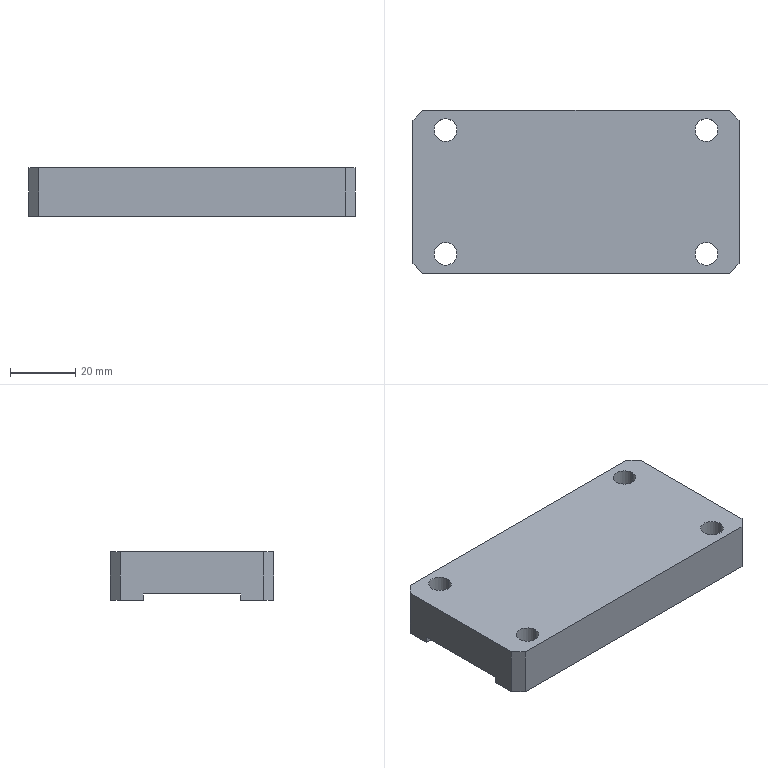Part | SolidWorks | features Chamfer 1, Extrusion 1, HoleWzd 1, ICE 1 | 1 solid | 22 faces | box 100 x 50 x 15 mm | volume 66421 mm3 | plane 14 | cylinder 8 | commonest cylinder face diameters 7 x8
STEP:
#1=CARTESIAN_POINT('',(13.5,44.,15.));
#2=VERTEX_POINT('',#1);
#3=CARTESIAN_POINT('',(6.5,44.,15.));
#4=VERTEX_POINT('',#3);
#5=CARTESIAN_POINT('',(10.,44.,15.));
#6=DIRECTION('',(0.,0.,-1.));
#7=DIRECTION('',(-1.,0.,0.));
#8=AXIS2_PLACEMENT_3D('',#5,#6,#7);
#9=CIRCLE('',#8,3.5);
#10=EDGE_CURVE('',#2,#4,#9,.T.);
#11=ORIENTED_EDGE('',*,*,#10,.F.);
#12=CARTESIAN_POINT('',(13.5,44.,0.));
#13=VERTEX_POINT('',#12);
#14=CARTESIAN_POINT('',(13.5,44.,0.));
#15=DIRECTION('',(0.,0.,-1.));
#16=VECTOR('',#15,1000.);
#17=LINE('',#14,#16);
#18=EDGE_CURVE('',#2,#13,#17,.T.);
#19=ORIENTED_EDGE('',*,*,#18,.T.);
#20=CARTESIAN_POINT('',(6.5,44.,0.));
#21=VERTEX_POINT('',#20);
#22=CARTESIAN_POINT('',(10.,44.,0.));
#23=DIRECTION('',(0.,0.,-1.));
#24=DIRECTION('',(-1.,0.,0.));
#25=AXIS2_PLACEMENT_3D('',#22,#23,#24);
#26=CIRCLE('',#25,3.5);
#27=EDGE_CURVE('',#13,#21,#26,.T.);
#28=ORIENTED_EDGE('',*,*,#27,.T.);
#29=CARTESIAN_POINT('',(6.5,44.,0.));
#30=DIRECTION('',(0.,0.,-1.));
#31=VECTOR('',#30,1000.);
#32=LINE('',#29,#31);
#33=EDGE_CURVE('',#4,#21,#32,.T.);
#34=ORIENTED_EDGE('',*,*,#33,.F.);
#35=EDGE_LOOP('',(#11,#19,#28,#34));
#36=FACE_OUTER_BOUND('',#35,.T.);
#37=CARTESIAN_POINT('',(10.,44.,0.));
#38=DIRECTION('',(0.,0.,-1.));
#39=DIRECTION('',(-1.,0.,0.));
#40=AXIS2_PLACEMENT_3D('',#37,#38,#39);
#41=CYLINDRICAL_SURFACE('',#40,3.5);
#42=ADVANCED_FACE('',(#36),#41,.F.);
#43=CARTESIAN_POINT('',(13.5,6.,15.));
#44=VERTEX_POINT('',#43);
#45=CARTESIAN_POINT('',(6.5,6.,15.));
#46=VERTEX_POINT('',#45);
#47=CARTESIAN_POINT('',(10.,6.,15.));
#48=DIRECTION('',(0.,0.,-1.));
#49=DIRECTION('',(-1.,0.,0.));
#50=AXIS2_PLACEMENT_3D('',#47,#48,#49);
#51=CIRCLE('',#50,3.5);
#52=EDGE_CURVE('',#44,#46,#51,.T.);
#53=ORIENTED_EDGE('',*,*,#52,.F.);
#54=CARTESIAN_POINT('',(13.5,6.,0.));
#55=VERTEX_POINT('',#54);
#56=CARTESIAN_POINT('',(13.5,6.,0.));
#57=DIRECTION('',(0.,0.,-1.));
#58=VECTOR('',#57,1000.);
#59=LINE('',#56,#58);
#60=EDGE_CURVE('',#44,#55,#59,.T.);
#61=ORIENTED_EDGE('',*,*,#60,.T.);
#62=CARTESIAN_POINT('',(6.5,6.,0.));
#63=VERTEX_POINT('',#62);
#64=CARTESIAN_POINT('',(10.,6.,0.));
#65=DIRECTION('',(0.,0.,-1.));
#66=DIRECTION('',(-1.,0.,0.));
#67=AXIS2_PLACEMENT_3D('',#64,#65,#66);
#68=CIRCLE('',#67,3.5);
#69=EDGE_CURVE('',#55,#63,#68,.T.);
#70=ORIENTED_EDGE('',*,*,#69,.T.);
#71=CARTESIAN_POINT('',(6.5,6.,0.));
#72=DIRECTION('',(0.,0.,-1.));
#73=VECTOR('',#72,1000.);
#74=LINE('',#71,#73);
#75=EDGE_CURVE('',#46,#63,#74,.T.);
#76=ORIENTED_EDGE('',*,*,#75,.F.);
#77=EDGE_LOOP('',(#53,#61,#70,#76));
#78=FACE_OUTER_BOUND('',#77,.T.);
#79=CARTESIAN_POINT('',(10.,6.,0.));
#80=DIRECTION('',(0.,0.,-1.));
#81=DIRECTION('',(-1.,0.,0.));
#82=AXIS2_PLACEMENT_3D('',#79,#80,#81);
#83=CYLINDRICAL_SURFACE('',#82,3.5);
#84=ADVANCED_FACE('',(#78),#83,.F.);
#85=CARTESIAN_POINT('',(93.5,44.,15.));
#86=VERTEX_POINT('',#85);
#87=CARTESIAN_POINT('',(86.5,44.,15.));
#88=VERTEX_POINT('',#87);
#89=CARTESIAN_POINT('',(90.,44.,15.));
#90=DIRECTION('',(0.,0.,-1.));
#91=DIRECTION('',(-1.,0.,0.));
#92=AXIS2_PLACEMENT_3D('',#89,#90,#91);
#93=CIRCLE('',#92,3.5);
#94=EDGE_CURVE('',#86,#88,#93,.T.);
#95=ORIENTED_EDGE('',*,*,#94,.F.);
#96=CARTESIAN_POINT('',(93.5,44.,0.));
#97=VERTEX_POINT('',#96);
#98=CARTESIAN_POINT('',(93.5,44.,0.));
#99=DIRECTION('',(0.,0.,-1.));
#100=VECTOR('',#99,1000.);
#101=LINE('',#98,#100);
#102=EDGE_CURVE('',#86,#97,#101,.T.);
#103=ORIENTED_EDGE('',*,*,#102,.T.);
#104=CARTESIAN_POINT('',(86.5,44.,0.));
#105=VERTEX_POINT('',#104);
#106=CARTESIAN_POINT('',(90.,44.,0.));
#107=DIRECTION('',(0.,0.,-1.));
#108=DIRECTION('',(-1.,0.,0.));
#109=AXIS2_PLACEMENT_3D('',#106,#107,#108);
#110=CIRCLE('',#109,3.5);
#111=EDGE_CURVE('',#97,#105,#110,.T.);
#112=ORIENTED_EDGE('',*,*,#111,.T.);
#113=CARTESIAN_POINT('',(86.5,44.,0.));
#114=DIRECTION('',(0.,0.,-1.));
#115=VECTOR('',#114,1000.);
#116=LINE('',#113,#115);
#117=EDGE_CURVE('',#88,#105,#116,.T.);
#118=ORIENTED_EDGE('',*,*,#117,.F.);
#119=EDGE_LOOP('',(#95,#103,#112,#118));
#120=FACE_OUTER_BOUND('',#119,.T.);
#121=CARTESIAN_POINT('',(90.,44.,0.));
#122=DIRECTION('',(0.,0.,-1.));
#123=DIRECTION('',(-1.,0.,0.));
#124=AXIS2_PLACEMENT_3D('',#121,#122,#123);
#125=CYLINDRICAL_SURFACE('',#124,3.5);
#126=ADVANCED_FACE('',(#120),#125,.F.);
#127=CARTESIAN_POINT('',(93.5,6.,15.));
#128=VERTEX_POINT('',#127);
#129=CARTESIAN_POINT('',(86.5,6.,15.));
#130=VERTEX_POINT('',#129);
#131=CARTESIAN_POINT('',(90.,6.,15.));
#132=DIRECTION('',(0.,0.,-1.));
#133=DIRECTION('',(-1.,0.,0.));
#134=AXIS2_PLACEMENT_3D('',#131,#132,#133);
#135=CIRCLE('',#134,3.5);
#136=EDGE_CURVE('',#128,#130,#135,.T.);
#137=ORIENTED_EDGE('',*,*,#136,.F.);
#138=CARTESIAN_POINT('',(93.5,6.,0.));
#139=VERTEX_POINT('',#138);
#140=CARTESIAN_POINT('',(93.5,6.,0.));
#141=DIRECTION('',(0.,0.,-1.));
#142=VECTOR('',#141,1000.);
#143=LINE('',#140,#142);
#144=EDGE_CURVE('',#128,#139,#143,.T.);
#145=ORIENTED_EDGE('',*,*,#144,.T.);
#146=CARTESIAN_POINT('',(86.5,6.,0.));
#147=VERTEX_POINT('',#146);
#148=CARTESIAN_POINT('',(90.,6.,0.));
#149=DIRECTION('',(0.,0.,-1.));
#150=DIRECTION('',(-1.,0.,0.));
#151=AXIS2_PLACEMENT_3D('',#148,#149,#150);
#152=CIRCLE('',#151,3.5);
#153=EDGE_CURVE('',#139,#147,#152,.T.);
#154=ORIENTED_EDGE('',*,*,#153,.T.);
#155=CARTESIAN_POINT('',(86.5,6.,0.));
#156=DIRECTION('',(0.,0.,-1.));
#157=VECTOR('',#156,1000.);
#158=LINE('',#155,#157);
#159=EDGE_CURVE('',#130,#147,#158,.T.);
#160=ORIENTED_EDGE('',*,*,#159,.F.);
#161=EDGE_LOOP('',(#137,#145,#154,#160));
#162=FACE_OUTER_BOUND('',#161,.T.);
#163=CARTESIAN_POINT('',(90.,6.,0.));
#164=DIRECTION('',(0.,0.,-1.));
#165=DIRECTION('',(-1.,0.,0.));
#166=AXIS2_PLACEMENT_3D('',#163,#164,#165);
#167=CYLINDRICAL_SURFACE('',#166,3.5);
#168=ADVANCED_FACE('',(#162),#167,.F.);
#169=CARTESIAN_POINT('',(0.,40.,0.));
#170=VERTEX_POINT('',#169);
#171=CARTESIAN_POINT('',(100.,40.,0.));
#172=VERTEX_POINT('',#171);
#173=CARTESIAN_POINT('',(0.,40.,0.));
#174=DIRECTION('',(1.,0.,0.));
#175=VECTOR('',#174,1000.);
#176=LINE('',#173,#175);
#177=EDGE_CURVE('',#170,#172,#176,.T.);
#178=ORIENTED_EDGE('',*,*,#177,.F.);
#179=CARTESIAN_POINT('',(0.,47.,0.));
#180=VERTEX_POINT('',#179);
#181=CARTESIAN_POINT('',(0.,0.,0.));
#182=DIRECTION('',(0.,-1.,0.));
#183=VECTOR('',#182,1000.);
#184=LINE('',#181,#183);
#185=EDGE_CURVE('',#180,#170,#184,.T.);
#186=ORIENTED_EDGE('',*,*,#185,.F.);
#187=CARTESIAN_POINT('',(3.,50.,0.));
#188=VERTEX_POINT('',#187);
#189=CARTESIAN_POINT('',(-23.5,23.5,0.));
#190=DIRECTION('',(0.7071,0.7071,0.));
#191=VECTOR('',#190,1000.);
#192=LINE('',#189,#191);
#193=EDGE_CURVE('',#180,#188,#192,.T.);
#194=ORIENTED_EDGE('',*,*,#193,.T.);
#195=CARTESIAN_POINT('',(97.,50.,0.));
#196=VERTEX_POINT('',#195);
#197=CARTESIAN_POINT('',(0.,50.,0.));
#198=DIRECTION('',(-1.,0.,0.));
#199=VECTOR('',#198,1000.);
#200=LINE('',#197,#199);
#201=EDGE_CURVE('',#196,#188,#200,.T.);
#202=ORIENTED_EDGE('',*,*,#201,.F.);
#203=CARTESIAN_POINT('',(100.,47.,0.));
#204=VERTEX_POINT('',#203);
#205=CARTESIAN_POINT('',(73.5,73.5,0.));
#206=DIRECTION('',(0.7071,-0.7071,0.));
#207=VECTOR('',#206,1000.);
#208=LINE('',#205,#207);
#209=EDGE_CURVE('',#196,#204,#208,.T.);
#210=ORIENTED_EDGE('',*,*,#209,.T.);
#211=CARTESIAN_POINT('',(100.,0.,0.));
#212=DIRECTION('',(0.,1.,0.));
#213=VECTOR('',#212,1000.);
#214=LINE('',#211,#213);
#215=EDGE_CURVE('',#172,#204,#214,.T.);
#216=ORIENTED_EDGE('',*,*,#215,.F.);
#217=EDGE_LOOP('',(#178,#186,#194,#202,#210,#216));
#218=FACE_OUTER_BOUND('',#217,.T.);
#219=CARTESIAN_POINT('',(90.,44.,0.));
#220=DIRECTION('',(0.,0.,-1.));
#221=DIRECTION('',(-1.,0.,0.));
#222=AXIS2_PLACEMENT_3D('',#219,#220,#221);
#223=CIRCLE('',#222,3.5);
#224=EDGE_CURVE('',#105,#97,#223,.T.);
#225=ORIENTED_EDGE('',*,*,#224,.F.);
#226=ORIENTED_EDGE('',*,*,#111,.F.);
#227=EDGE_LOOP('',(#225,#226));
#228=FACE_BOUND('',#227,.T.);
#229=CARTESIAN_POINT('',(10.,44.,0.));
#230=DIRECTION('',(0.,0.,-1.));
#231=DIRECTION('',(-1.,0.,0.));
#232=AXIS2_PLACEMENT_3D('',#229,#230,#231);
#233=CIRCLE('',#232,3.5);
#234=EDGE_CURVE('',#21,#13,#233,.T.);
#235=ORIENTED_EDGE('',*,*,#234,.F.);
#236=ORIENTED_EDGE('',*,*,#27,.F.);
#237=EDGE_LOOP('',(#235,#236));
#238=FACE_BOUND('',#237,.T.);
#239=CARTESIAN_POINT('',(0.,0.,0.));
#240=DIRECTION('',(0.,0.,-1.));
#241=DIRECTION('',(-1.,0.,0.));
#242=AXIS2_PLACEMENT_3D('',#239,#240,#241);
#243=PLANE('',#242);
#244=ADVANCED_FACE('',(#218,#228,#238),#243,.T.);
#245=ORIENTED_EDGE('',*,*,#185,.T.);
#246=CARTESIAN_POINT('',(0.,40.,2.));
#247=VERTEX_POINT('',#246);
#248=CARTESIAN_POINT('',(0.,40.,0.));
#249=DIRECTION('',(0.,0.,-1.));
#250=VECTOR('',#249,1000.);
#251=LINE('',#248,#250);
#252=EDGE_CURVE('',#247,#170,#251,.T.);
#253=ORIENTED_EDGE('',*,*,#252,.F.);
#254=CARTESIAN_POINT('',(0.,10.,2.));
#255=VERTEX_POINT('',#254);
#256=CARTESIAN_POINT('',(0.,40.,2.));
#257=DIRECTION('',(0.,1.,0.));
#258=VECTOR('',#257,1000.);
#259=LINE('',#256,#258);
#260=EDGE_CURVE('',#255,#247,#259,.T.);
#261=ORIENTED_EDGE('',*,*,#260,.F.);
#262=CARTESIAN_POINT('',(0.,10.,0.));
#263=VERTEX_POINT('',#262);
#264=CARTESIAN_POINT('',(0.,10.,0.));
#265=DIRECTION('',(0.,0.,1.));
#266=VECTOR('',#265,1000.);
#267=LINE('',#264,#266);
#268=EDGE_CURVE('',#263,#255,#267,.T.);
#269=ORIENTED_EDGE('',*,*,#268,.F.);
#270=CARTESIAN_POINT('',(0.,3.,0.));
#271=VERTEX_POINT('',#270);
#272=CARTESIAN_POINT('',(0.,0.,0.));
#273=DIRECTION('',(0.,-1.,0.));
#274=VECTOR('',#273,1000.);
#275=LINE('',#272,#274);
#276=EDGE_CURVE('',#263,#271,#275,.T.);
#277=ORIENTED_EDGE('',*,*,#276,.T.);
#278=CARTESIAN_POINT('',(0.,3.,15.));
#279=VERTEX_POINT('',#278);
#280=CARTESIAN_POINT('',(0.,3.,15.));
#281=DIRECTION('',(0.,0.,1.));
#282=VECTOR('',#281,1000.);
#283=LINE('',#280,#282);
#284=EDGE_CURVE('',#271,#279,#283,.T.);
#285=ORIENTED_EDGE('',*,*,#284,.T.);
#286=CARTESIAN_POINT('',(0.,47.,15.));
#287=VERTEX_POINT('',#286);
#288=CARTESIAN_POINT('',(0.,0.,15.));
#289=DIRECTION('',(0.,-1.,0.));
#290=VECTOR('',#289,1000.);
#291=LINE('',#288,#290);
#292=EDGE_CURVE('',#287,#279,#291,.T.);
#293=ORIENTED_EDGE('',*,*,#292,.F.);
#294=CARTESIAN_POINT('',(0.,47.,15.));
#295=DIRECTION('',(0.,0.,-1.));
#296=VECTOR('',#295,1000.);
#297=LINE('',#294,#296);
#298=EDGE_CURVE('',#287,#180,#297,.T.);
#299=ORIENTED_EDGE('',*,*,#298,.T.);
#300=EDGE_LOOP('',(#245,#253,#261,#269,#277,#285,#293,#299));
#301=FACE_OUTER_BOUND('',#300,.T.);
#302=CARTESIAN_POINT('',(0.,0.,15.));
#303=DIRECTION('',(1.,0.,0.));
#304=DIRECTION('',(0.,0.,-1.));
#305=AXIS2_PLACEMENT_3D('',#302,#303,#304);
#306=PLANE('',#305);
#307=ADVANCED_FACE('',(#301),#306,.F.);
#308=CARTESIAN_POINT('',(3.,0.,15.));
#309=VERTEX_POINT('',#308);
#310=CARTESIAN_POINT('',(97.,0.,15.));
#311=VERTEX_POINT('',#310);
#312=CARTESIAN_POINT('',(0.,0.,15.));
#313=DIRECTION('',(1.,0.,0.));
#314=VECTOR('',#313,1000.);
#315=LINE('',#312,#314);
#316=EDGE_CURVE('',#309,#311,#315,.T.);
#317=ORIENTED_EDGE('',*,*,#316,.F.);
#318=CARTESIAN_POINT('',(3.,0.,0.));
#319=VERTEX_POINT('',#318);
#320=CARTESIAN_POINT('',(3.,0.,15.));
#321=DIRECTION('',(0.,0.,-1.));
#322=VECTOR('',#321,1000.);
#323=LINE('',#320,#322);
#324=EDGE_CURVE('',#309,#319,#323,.T.);
#325=ORIENTED_EDGE('',*,*,#324,.T.);
#326=CARTESIAN_POINT('',(97.,0.,0.));
#327=VERTEX_POINT('',#326);
#328=CARTESIAN_POINT('',(0.,0.,0.));
#329=DIRECTION('',(1.,0.,0.));
#330=VECTOR('',#329,1000.);
#331=LINE('',#328,#330);
#332=EDGE_CURVE('',#319,#327,#331,.T.);
#333=ORIENTED_EDGE('',*,*,#332,.T.);
#334=CARTESIAN_POINT('',(97.,0.,15.));
#335=DIRECTION('',(0.,0.,1.));
#336=VECTOR('',#335,1000.);
#337=LINE('',#334,#336);
#338=EDGE_CURVE('',#327,#311,#337,.T.);
#339=ORIENTED_EDGE('',*,*,#338,.T.);
#340=EDGE_LOOP('',(#317,#325,#333,#339));
#341=FACE_OUTER_BOUND('',#340,.T.);
#342=CARTESIAN_POINT('',(0.,0.,15.));
#343=DIRECTION('',(0.,1.,0.));
#344=DIRECTION('',(0.,0.,1.));
#345=AXIS2_PLACEMENT_3D('',#342,#343,#344);
#346=PLANE('',#345);
#347=ADVANCED_FACE('',(#341),#346,.F.);
#348=CARTESIAN_POINT('',(100.,10.,2.));
#349=VERTEX_POINT('',#348);
#350=CARTESIAN_POINT('',(100.,40.,2.));
#351=VERTEX_POINT('',#350);
#352=CARTESIAN_POINT('',(100.,0.,2.));
#353=DIRECTION('',(0.,1.,0.));
#354=VECTOR('',#353,1000.);
#355=LINE('',#352,#354);
#356=EDGE_CURVE('',#349,#351,#355,.T.);
#357=ORIENTED_EDGE('',*,*,#356,.T.);
#358=CARTESIAN_POINT('',(100.,40.,15.));
#359=DIRECTION('',(0.,0.,-1.));
#360=VECTOR('',#359,1000.);
#361=LINE('',#358,#360);
#362=EDGE_CURVE('',#351,#172,#361,.T.);
#363=ORIENTED_EDGE('',*,*,#362,.T.);
#364=ORIENTED_EDGE('',*,*,#215,.T.);
#365=CARTESIAN_POINT('',(100.,47.,15.));
#366=VERTEX_POINT('',#365);
#367=CARTESIAN_POINT('',(100.,47.,15.));
#368=DIRECTION('',(0.,0.,1.));
#369=VECTOR('',#368,1000.);
#370=LINE('',#367,#369);
#371=EDGE_CURVE('',#204,#366,#370,.T.);
#372=ORIENTED_EDGE('',*,*,#371,.T.);
#373=CARTESIAN_POINT('',(100.,3.,15.));
#374=VERTEX_POINT('',#373);
#375=CARTESIAN_POINT('',(100.,0.,15.));
#376=DIRECTION('',(0.,1.,0.));
#377=VECTOR('',#376,1000.);
#378=LINE('',#375,#377);
#379=EDGE_CURVE('',#374,#366,#378,.T.);
#380=ORIENTED_EDGE('',*,*,#379,.F.);
#381=CARTESIAN_POINT('',(100.,3.,0.));
#382=VERTEX_POINT('',#381);
#383=CARTESIAN_POINT('',(100.,3.,15.));
#384=DIRECTION('',(0.,0.,-1.));
#385=VECTOR('',#384,1000.);
#386=LINE('',#383,#385);
#387=EDGE_CURVE('',#374,#382,#386,.T.);
#388=ORIENTED_EDGE('',*,*,#387,.T.);
#389=CARTESIAN_POINT('',(100.,10.,0.));
#390=VERTEX_POINT('',#389);
#391=CARTESIAN_POINT('',(100.,0.,0.));
#392=DIRECTION('',(0.,1.,0.));
#393=VECTOR('',#392,1000.);
#394=LINE('',#391,#393);
#395=EDGE_CURVE('',#382,#390,#394,.T.);
#396=ORIENTED_EDGE('',*,*,#395,.T.);
#397=CARTESIAN_POINT('',(100.,10.,15.));
#398=DIRECTION('',(0.,0.,1.));
#399=VECTOR('',#398,1000.);
#400=LINE('',#397,#399);
#401=EDGE_CURVE('',#390,#349,#400,.T.);
#402=ORIENTED_EDGE('',*,*,#401,.T.);
#403=EDGE_LOOP('',(#357,#363,#364,#372,#380,#388,#396,#402));
#404=FACE_OUTER_BOUND('',#403,.T.);
#405=CARTESIAN_POINT('',(100.,0.,15.));
#406=DIRECTION('',(-1.,0.,0.));
#407=DIRECTION('',(0.,0.,1.));
#408=AXIS2_PLACEMENT_3D('',#405,#406,#407);
#409=PLANE('',#408);
#410=ADVANCED_FACE('',(#404),#409,.F.);
#411=ORIENTED_EDGE('',*,*,#201,.T.);
#412=CARTESIAN_POINT('',(3.,50.,15.));
#413=VERTEX_POINT('',#412);
#414=CARTESIAN_POINT('',(3.,50.,15.));
#415=DIRECTION('',(0.,0.,1.));
#416=VECTOR('',#415,1000.);
#417=LINE('',#414,#416);
#418=EDGE_CURVE('',#188,#413,#417,.T.);
#419=ORIENTED_EDGE('',*,*,#418,.T.);
#420=CARTESIAN_POINT('',(97.,50.,15.));
#421=VERTEX_POINT('',#420);
#422=CARTESIAN_POINT('',(0.,50.,15.));
#423=DIRECTION('',(-1.,0.,0.));
#424=VECTOR('',#423,1000.);
#425=LINE('',#422,#424);
#426=EDGE_CURVE('',#421,#413,#425,.T.);
#427=ORIENTED_EDGE('',*,*,#426,.F.);
#428=CARTESIAN_POINT('',(97.,50.,15.));
#429=DIRECTION('',(0.,0.,-1.));
#430=VECTOR('',#429,1000.);
#431=LINE('',#428,#430);
#432=EDGE_CURVE('',#421,#196,#431,.T.);
#433=ORIENTED_EDGE('',*,*,#432,.T.);
#434=EDGE_LOOP('',(#411,#419,#427,#433));
#435=FACE_OUTER_BOUND('',#434,.T.);
#436=CARTESIAN_POINT('',(0.,50.,15.));
#437=DIRECTION('',(0.,-1.,0.));
#438=DIRECTION('',(0.,0.,-1.));
#439=AXIS2_PLACEMENT_3D('',#436,#437,#438);
#440=PLANE('',#439);
#441=ADVANCED_FACE('',(#435),#440,.F.);
#442=CARTESIAN_POINT('',(10.,44.,15.));
#443=DIRECTION('',(0.,0.,-1.));
#444=DIRECTION('',(-1.,0.,0.));
#445=AXIS2_PLACEMENT_3D('',#442,#443,#444);
#446=CIRCLE('',#445,3.5);
#447=EDGE_CURVE('',#4,#2,#446,.T.);
#448=ORIENTED_EDGE('',*,*,#447,.T.);
#449=ORIENTED_EDGE('',*,*,#10,.T.);
#450=EDGE_LOOP('',(#448,#449));
#451=FACE_BOUND('',#450,.T.);
#452=CARTESIAN_POINT('',(10.,6.,15.));
#453=DIRECTION('',(0.,0.,-1.));
#454=DIRECTION('',(-1.,0.,0.));
#455=AXIS2_PLACEMENT_3D('',#452,#453,#454);
#456=CIRCLE('',#455,3.5);
#457=EDGE_CURVE('',#46,#44,#456,.T.);
#458=ORIENTED_EDGE('',*,*,#457,.T.);
#459=ORIENTED_EDGE('',*,*,#52,.T.);
#460=EDGE_LOOP('',(#458,#459));
#461=FACE_BOUND('',#460,.T.);
#462=CARTESIAN_POINT('',(90.,44.,15.));
#463=DIRECTION('',(0.,0.,-1.));
#464=DIRECTION('',(-1.,0.,0.));
#465=AXIS2_PLACEMENT_3D('',#462,#463,#464);
#466=CIRCLE('',#465,3.5);
#467=EDGE_CURVE('',#88,#86,#466,.T.);
#468=ORIENTED_EDGE('',*,*,#467,.T.);
#469=ORIENTED_EDGE('',*,*,#94,.T.);
#470=EDGE_LOOP('',(#468,#469));
#471=FACE_BOUND('',#470,.T.);
#472=CARTESIAN_POINT('',(90.,6.,15.));
#473=DIRECTION('',(0.,0.,-1.));
#474=DIRECTION('',(-1.,0.,0.));
#475=AXIS2_PLACEMENT_3D('',#472,#473,#474);
#476=CIRCLE('',#475,3.5);
#477=EDGE_CURVE('',#130,#128,#476,.T.);
#478=ORIENTED_EDGE('',*,*,#477,.T.);
#479=ORIENTED_EDGE('',*,*,#136,.T.);
#480=EDGE_LOOP('',(#478,#479));
#481=FACE_BOUND('',#480,.T.);
#482=ORIENTED_EDGE('',*,*,#292,.T.);
#483=CARTESIAN_POINT('',(3.,0.,15.));
#484=DIRECTION('',(0.7071,-0.7071,0.));
#485=VECTOR('',#484,1000.);
#486=LINE('',#483,#485);
#487=EDGE_CURVE('',#279,#309,#486,.T.);
#488=ORIENTED_EDGE('',*,*,#487,.T.);
#489=ORIENTED_EDGE('',*,*,#316,.T.);
#490=CARTESIAN_POINT('',(100.,3.,15.));
#491=DIRECTION('',(0.7071,0.7071,0.));
#492=VECTOR('',#491,1000.);
#493=LINE('',#490,#492);
#494=EDGE_CURVE('',#311,#374,#493,.T.);
#495=ORIENTED_EDGE('',*,*,#494,.T.);
#496=ORIENTED_EDGE('',*,*,#379,.T.);
#497=CARTESIAN_POINT('',(97.,50.,15.));
#498=DIRECTION('',(-0.7071,0.7071,0.));
#499=VECTOR('',#498,1000.);
#500=LINE('',#497,#499);
#501=EDGE_CURVE('',#366,#421,#500,.T.);
#502=ORIENTED_EDGE('',*,*,#501,.T.);
#503=ORIENTED_EDGE('',*,*,#426,.T.);
#504=CARTESIAN_POINT('',(0.,47.,15.));
#505=DIRECTION('',(-0.7071,-0.7071,0.));
#506=VECTOR('',#505,1000.);
#507=LINE('',#504,#506);
#508=EDGE_CURVE('',#413,#287,#507,.T.);
#509=ORIENTED_EDGE('',*,*,#508,.T.);
#510=EDGE_LOOP('',(#482,#488,#489,#495,#496,#502,#503,#509));
#511=FACE_OUTER_BOUND('',#510,.T.);
#512=CARTESIAN_POINT('',(0.,0.,15.));
#513=DIRECTION('',(0.,0.,-1.));
#514=DIRECTION('',(-1.,0.,0.));
#515=AXIS2_PLACEMENT_3D('',#512,#513,#514);
#516=PLANE('',#515);
#517=ADVANCED_FACE('',(#451,#461,#471,#481,#511),#516,.F.);
#518=CARTESIAN_POINT('',(0.,10.,0.));
#519=DIRECTION('',(-1.,0.,0.));
#520=VECTOR('',#519,1000.);
#521=LINE('',#518,#520);
#522=EDGE_CURVE('',#390,#263,#521,.T.);
#523=ORIENTED_EDGE('',*,*,#522,.F.);
#524=ORIENTED_EDGE('',*,*,#395,.F.);
#525=CARTESIAN_POINT('',(48.5,-48.5,0.));
#526=DIRECTION('',(-0.7071,-0.7071,0.));
#527=VECTOR('',#526,1000.);
#528=LINE('',#525,#527);
#529=EDGE_CURVE('',#382,#327,#528,.T.);
#530=ORIENTED_EDGE('',*,*,#529,.T.);
#531=ORIENTED_EDGE('',*,*,#332,.F.);
#532=CARTESIAN_POINT('',(1.5,1.5,0.));
#533=DIRECTION('',(-0.7071,0.7071,0.));
#534=VECTOR('',#533,1000.);
#535=LINE('',#532,#534);
#536=EDGE_CURVE('',#319,#271,#535,.T.);
#537=ORIENTED_EDGE('',*,*,#536,.T.);
#538=ORIENTED_EDGE('',*,*,#276,.F.);
#539=EDGE_LOOP('',(#523,#524,#530,#531,#537,#538));
#540=FACE_OUTER_BOUND('',#539,.T.);
#541=CARTESIAN_POINT('',(10.,6.,0.));
#542=DIRECTION('',(0.,0.,-1.));
#543=DIRECTION('',(-1.,0.,0.));
#544=AXIS2_PLACEMENT_3D('',#541,#542,#543);
#545=CIRCLE('',#544,3.5);
#546=EDGE_CURVE('',#63,#55,#545,.T.);
#547=ORIENTED_EDGE('',*,*,#546,.F.);
#548=ORIENTED_EDGE('',*,*,#69,.F.);
#549=EDGE_LOOP('',(#547,#548));
#550=FACE_BOUND('',#549,.T.);
#551=CARTESIAN_POINT('',(90.,6.,0.));
#552=DIRECTION('',(0.,0.,-1.));
#553=DIRECTION('',(-1.,0.,0.));
#554=AXIS2_PLACEMENT_3D('',#551,#552,#553);
#555=CIRCLE('',#554,3.5);
#556=EDGE_CURVE('',#147,#139,#555,.T.);
#557=ORIENTED_EDGE('',*,*,#556,.F.);
#558=ORIENTED_EDGE('',*,*,#153,.F.);
#559=EDGE_LOOP('',(#557,#558));
#560=FACE_BOUND('',#559,.T.);
#561=CARTESIAN_POINT('',(0.,0.,0.));
#562=DIRECTION('',(0.,0.,-1.));
#563=DIRECTION('',(-1.,0.,0.));
#564=AXIS2_PLACEMENT_3D('',#561,#562,#563);
#565=PLANE('',#564);
#566=ADVANCED_FACE('',(#540,#550,#560),#565,.T.);
#567=ORIENTED_EDGE('',*,*,#144,.F.);
#568=ORIENTED_EDGE('',*,*,#477,.F.);
#569=ORIENTED_EDGE('',*,*,#159,.T.);
#570=ORIENTED_EDGE('',*,*,#556,.T.);
#571=EDGE_LOOP('',(#567,#568,#569,#570));
#572=FACE_OUTER_BOUND('',#571,.T.);
#573=CARTESIAN_POINT('',(90.,6.,0.));
#574=DIRECTION('',(0.,0.,-1.));
#575=DIRECTION('',(-1.,0.,0.));
#576=AXIS2_PLACEMENT_3D('',#573,#574,#575);
#577=CYLINDRICAL_SURFACE('',#576,3.5);
#578=ADVANCED_FACE('',(#572),#577,.F.);
#579=ORIENTED_EDGE('',*,*,#102,.F.);
#580=ORIENTED_EDGE('',*,*,#467,.F.);
#581=ORIENTED_EDGE('',*,*,#117,.T.);
#582=ORIENTED_EDGE('',*,*,#224,.T.);
#583=EDGE_LOOP('',(#579,#580,#581,#582));
#584=FACE_OUTER_BOUND('',#583,.T.);
#585=CARTESIAN_POINT('',(90.,44.,0.));
#586=DIRECTION('',(0.,0.,-1.));
#587=DIRECTION('',(-1.,0.,0.));
#588=AXIS2_PLACEMENT_3D('',#585,#586,#587);
#589=CYLINDRICAL_SURFACE('',#588,3.5);
#590=ADVANCED_FACE('',(#584),#589,.F.);
#591=ORIENTED_EDGE('',*,*,#60,.F.);
#592=ORIENTED_EDGE('',*,*,#457,.F.);
#593=ORIENTED_EDGE('',*,*,#75,.T.);
#594=ORIENTED_EDGE('',*,*,#546,.T.);
#595=EDGE_LOOP('',(#591,#592,#593,#594));
#596=FACE_OUTER_BOUND('',#595,.T.);
#597=CARTESIAN_POINT('',(10.,6.,0.));
#598=DIRECTION('',(0.,0.,-1.));
#599=DIRECTION('',(-1.,0.,0.));
#600=AXIS2_PLACEMENT_3D('',#597,#598,#599);
#601=CYLINDRICAL_SURFACE('',#600,3.5);
#602=ADVANCED_FACE('',(#596),#601,.F.);
#603=ORIENTED_EDGE('',*,*,#18,.F.);
#604=ORIENTED_EDGE('',*,*,#447,.F.);
#605=ORIENTED_EDGE('',*,*,#33,.T.);
#606=ORIENTED_EDGE('',*,*,#234,.T.);
#607=EDGE_LOOP('',(#603,#604,#605,#606));
#608=FACE_OUTER_BOUND('',#607,.T.);
#609=CARTESIAN_POINT('',(10.,44.,0.));
#610=DIRECTION('',(0.,0.,-1.));
#611=DIRECTION('',(-1.,0.,0.));
#612=AXIS2_PLACEMENT_3D('',#609,#610,#611);
#613=CYLINDRICAL_SURFACE('',#612,3.5);
#614=ADVANCED_FACE('',(#608),#613,.F.);
#615=ORIENTED_EDGE('',*,*,#487,.F.);
#616=ORIENTED_EDGE('',*,*,#284,.F.);
#617=ORIENTED_EDGE('',*,*,#536,.F.);
#618=ORIENTED_EDGE('',*,*,#324,.F.);
#619=EDGE_LOOP('',(#615,#616,#617,#618));
#620=FACE_OUTER_BOUND('',#619,.T.);
#621=CARTESIAN_POINT('',(3.,0.,15.));
#622=DIRECTION('',(0.7071,0.7071,0.));
#623=DIRECTION('',(0.,0.,-1.));
#624=AXIS2_PLACEMENT_3D('',#621,#622,#623);
#625=PLANE('',#624);
#626=ADVANCED_FACE('',(#620),#625,.F.);
#627=ORIENTED_EDGE('',*,*,#508,.F.);
#628=ORIENTED_EDGE('',*,*,#418,.F.);
#629=ORIENTED_EDGE('',*,*,#193,.F.);
#630=ORIENTED_EDGE('',*,*,#298,.F.);
#631=EDGE_LOOP('',(#627,#628,#629,#630));
#632=FACE_OUTER_BOUND('',#631,.T.);
#633=CARTESIAN_POINT('',(0.,47.,15.));
#634=DIRECTION('',(0.7071,-0.7071,0.));
#635=DIRECTION('',(0.,0.,-1.));
#636=AXIS2_PLACEMENT_3D('',#633,#634,#635);
#637=PLANE('',#636);
#638=ADVANCED_FACE('',(#632),#637,.F.);
#639=ORIENTED_EDGE('',*,*,#494,.F.);
#640=ORIENTED_EDGE('',*,*,#338,.F.);
#641=ORIENTED_EDGE('',*,*,#529,.F.);
#642=ORIENTED_EDGE('',*,*,#387,.F.);
#643=EDGE_LOOP('',(#639,#640,#641,#642));
#644=FACE_OUTER_BOUND('',#643,.T.);
#645=CARTESIAN_POINT('',(100.,3.,15.));
#646=DIRECTION('',(-0.7071,0.7071,0.));
#647=DIRECTION('',(0.,0.,-1.));
#648=AXIS2_PLACEMENT_3D('',#645,#646,#647);
#649=PLANE('',#648);
#650=ADVANCED_FACE('',(#644),#649,.F.);
#651=ORIENTED_EDGE('',*,*,#501,.F.);
#652=ORIENTED_EDGE('',*,*,#371,.F.);
#653=ORIENTED_EDGE('',*,*,#209,.F.);
#654=ORIENTED_EDGE('',*,*,#432,.F.);
#655=EDGE_LOOP('',(#651,#652,#653,#654));
#656=FACE_OUTER_BOUND('',#655,.T.);
#657=CARTESIAN_POINT('',(97.,50.,15.));
#658=DIRECTION('',(-0.7071,-0.7071,0.));
#659=DIRECTION('',(0.,0.,-1.));
#660=AXIS2_PLACEMENT_3D('',#657,#658,#659);
#661=PLANE('',#660);
#662=ADVANCED_FACE('',(#656),#661,.F.);
#663=CARTESIAN_POINT('',(113.,10.,2.));
#664=DIRECTION('',(-1.,0.,0.));
#665=VECTOR('',#664,1000.);
#666=LINE('',#663,#665);
#667=EDGE_CURVE('',#349,#255,#666,.T.);
#668=ORIENTED_EDGE('',*,*,#667,.T.);
#669=ORIENTED_EDGE('',*,*,#260,.T.);
#670=CARTESIAN_POINT('',(113.,40.,2.));
#671=DIRECTION('',(-1.,0.,0.));
#672=VECTOR('',#671,1000.);
#673=LINE('',#670,#672);
#674=EDGE_CURVE('',#351,#247,#673,.T.);
#675=ORIENTED_EDGE('',*,*,#674,.F.);
#676=ORIENTED_EDGE('',*,*,#356,.F.);
#677=EDGE_LOOP('',(#668,#669,#675,#676));
#678=FACE_OUTER_BOUND('',#677,.T.);
#679=CARTESIAN_POINT('',(113.,40.,2.));
#680=DIRECTION('',(0.,0.,1.));
#681=DIRECTION('',(0.,-1.,0.));
#682=AXIS2_PLACEMENT_3D('',#679,#680,#681);
#683=PLANE('',#682);
#684=ADVANCED_FACE('',(#678),#683,.F.);
#685=ORIENTED_EDGE('',*,*,#674,.T.);
#686=ORIENTED_EDGE('',*,*,#252,.T.);
#687=ORIENTED_EDGE('',*,*,#177,.T.);
#688=ORIENTED_EDGE('',*,*,#362,.F.);
#689=EDGE_LOOP('',(#685,#686,#687,#688));
#690=FACE_OUTER_BOUND('',#689,.T.);
#691=CARTESIAN_POINT('',(113.,40.,0.));
#692=DIRECTION('',(0.,1.,0.));
#693=DIRECTION('',(0.,0.,1.));
#694=AXIS2_PLACEMENT_3D('',#691,#692,#693);
#695=PLANE('',#694);
#696=ADVANCED_FACE('',(#690),#695,.F.);
#697=ORIENTED_EDGE('',*,*,#522,.T.);
#698=ORIENTED_EDGE('',*,*,#268,.T.);
#699=ORIENTED_EDGE('',*,*,#667,.F.);
#700=ORIENTED_EDGE('',*,*,#401,.F.);
#701=EDGE_LOOP('',(#697,#698,#699,#700));
#702=FACE_OUTER_BOUND('',#701,.T.);
#703=CARTESIAN_POINT('',(113.,10.,0.));
#704=DIRECTION('',(0.,-1.,0.));
#705=DIRECTION('',(0.,0.,-1.));
#706=AXIS2_PLACEMENT_3D('',#703,#704,#705);
#707=PLANE('',#706);
#708=ADVANCED_FACE('',(#702),#707,.F.);
#709=CLOSED_SHELL('',(#42,#84,#126,#168,#244,#307,#347,#410,#441,#517,#566,#578,#590,#602,#614,#626,#638,#650,#662,#684,#696,#708));
#710=MANIFOLD_SOLID_BREP('',#709);
#711=CARTESIAN_POINT('',(0.,0.,0.));
#712=DIRECTION('',(0.,0.,1.));
#713=DIRECTION('',(1.,0.,0.));
#714=AXIS2_PLACEMENT_3D('',#711,#712,#713);
#715=(LENGTH_UNIT()NAMED_UNIT(*)SI_UNIT(.MILLI.,.METRE.));
#716=UNCERTAINTY_MEASURE_WITH_UNIT(LENGTH_MEASURE(0.00001),#715,'','');
#717=(NAMED_UNIT(*)PLANE_ANGLE_UNIT()SI_UNIT($,.RADIAN.));
#718=(NAMED_UNIT(*)SI_UNIT($,.STERADIAN.)SOLID_ANGLE_UNIT());
#719=(GEOMETRIC_REPRESENTATION_CONTEXT(3)GLOBAL_UNCERTAINTY_ASSIGNED_CONTEXT((#716))GLOBAL_UNIT_ASSIGNED_CONTEXT((#715,#717,#718))REPRESENTATION_CONTEXT('',''));
#720=ADVANCED_BREP_SHAPE_REPRESENTATION('',(#710,#714),#719);